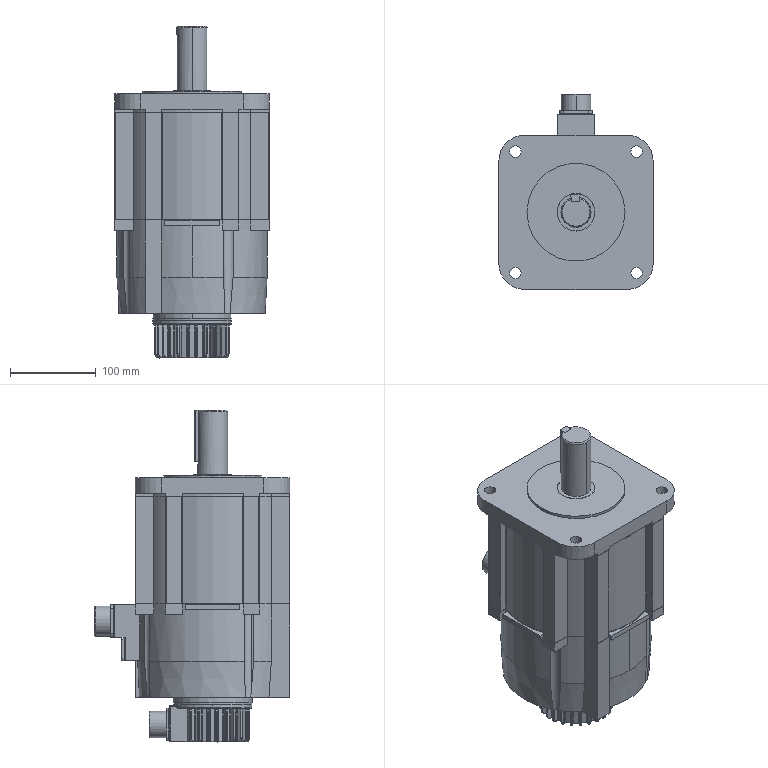Part | SolidWorks | features BaseBody 19 | 19 solids | 1044 faces | box 180 x 228 x 387 mm | volume 7070926 mm3 | cylinder 488 | spline 278 | plane 258 | cone 20 | commonest cylinder face diameters 2 x178 1 x38 1.8 x34 3 x30 175 x27 10 x23